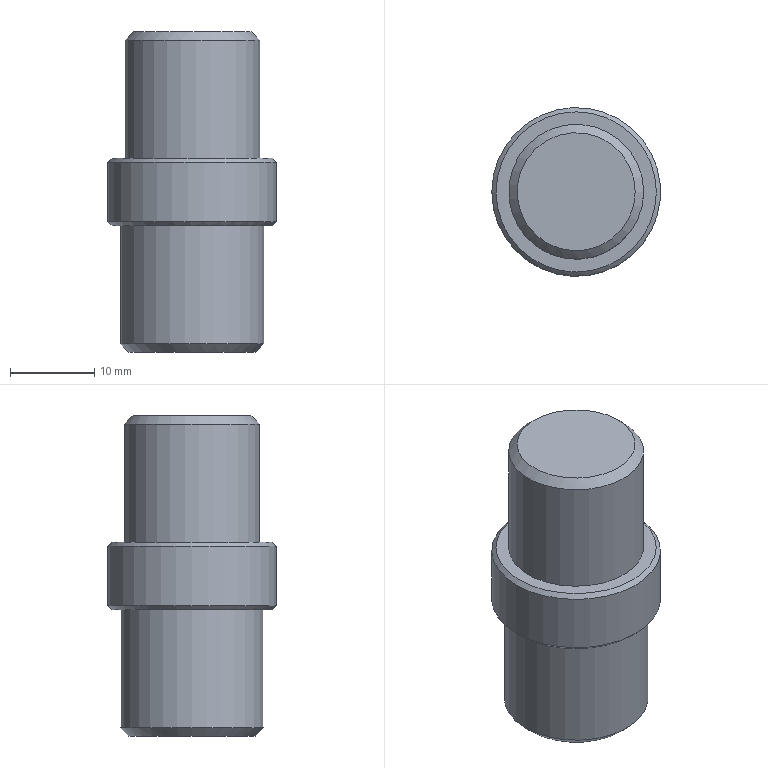Part | NX | features DATUM_CSYS 4, EXTRUDE 3, SKETCH 3, CHAMFER 2 | 1 solid | 11 faces | box 20 x 20 x 38 mm | volume 8869 mm3 | plane 4 | cone 4 | cylinder 3 | commonest cylinder face diameters 16 x1 17 x1 20 x1
STEP:
#1=CARTESIAN_POINT('',(8.,0.,14.));
#2=VERTEX_POINT('',#1);
#3=CARTESIAN_POINT('',(0.,0.,14.));
#4=DIRECTION('',(0.,0.,1.));
#5=DIRECTION('',(1.,0.,0.));
#6=AXIS2_PLACEMENT_3D('',#3,#4,#5);
#7=CIRCLE('',#6,8.);
#8=EDGE_CURVE('',#2,#2,#7,.F.);
#9=ORIENTED_EDGE('',*,*,#8,.T.);
#10=EDGE_LOOP('',(#9));
#11=FACE_BOUND('',#10,.T.);
#12=CARTESIAN_POINT('',(8.,0.,0.));
#13=VERTEX_POINT('',#12);
#14=CARTESIAN_POINT('',(0.,0.,0.));
#15=DIRECTION('',(0.,0.,1.));
#16=DIRECTION('',(1.,0.,0.));
#17=AXIS2_PLACEMENT_3D('',#14,#15,#16);
#18=CIRCLE('',#17,8.);
#19=EDGE_CURVE('',#13,#13,#18,.T.);
#20=ORIENTED_EDGE('',*,*,#19,.T.);
#21=EDGE_LOOP('',(#20));
#22=FACE_BOUND('',#21,.T.);
#23=CARTESIAN_POINT('',(0.,0.,15.));
#24=DIRECTION('',(0.,0.,-1.));
#25=DIRECTION('',(-1.,0.,0.));
#26=AXIS2_PLACEMENT_3D('',#23,#24,#25);
#27=CYLINDRICAL_SURFACE('',#26,8.);
#28=ADVANCED_FACE('',(#11,#22),#27,.T.);
#29=CARTESIAN_POINT('',(7.,0.,15.));
#30=VERTEX_POINT('',#29);
#31=CARTESIAN_POINT('',(0.,0.,15.));
#32=DIRECTION('',(0.,0.,1.));
#33=DIRECTION('',(1.,0.,0.));
#34=AXIS2_PLACEMENT_3D('',#31,#32,#33);
#35=CIRCLE('',#34,7.);
#36=EDGE_CURVE('',#30,#30,#35,.T.);
#37=ORIENTED_EDGE('',*,*,#36,.T.);
#38=EDGE_LOOP('',(#37));
#39=FACE_BOUND('',#38,.T.);
#40=CARTESIAN_POINT('',(0.,0.,15.));
#41=DIRECTION('',(0.,0.,1.));
#42=DIRECTION('',(1.,0.,0.));
#43=AXIS2_PLACEMENT_3D('',#40,#41,#42);
#44=PLANE('',#43);
#45=ADVANCED_FACE('',(#39),#44,.T.);
#46=CARTESIAN_POINT('',(-10.,0.,-7.5));
#47=VERTEX_POINT('',#46);
#48=CARTESIAN_POINT('',(0.,0.,-7.5));
#49=DIRECTION('',(0.,0.,-1.));
#50=DIRECTION('',(-1.,0.,0.));
#51=AXIS2_PLACEMENT_3D('',#48,#49,#50);
#52=CIRCLE('',#51,10.);
#53=EDGE_CURVE('',#47,#47,#52,.F.);
#54=ORIENTED_EDGE('',*,*,#53,.T.);
#55=EDGE_LOOP('',(#54));
#56=FACE_BOUND('',#55,.T.);
#57=CARTESIAN_POINT('',(-10.,0.,-0.5));
#58=VERTEX_POINT('',#57);
#59=CARTESIAN_POINT('',(0.,0.,-0.5));
#60=DIRECTION('',(0.,0.,-1.));
#61=DIRECTION('',(-1.,0.,0.));
#62=AXIS2_PLACEMENT_3D('',#59,#60,#61);
#63=CIRCLE('',#62,10.);
#64=EDGE_CURVE('',#58,#58,#63,.T.);
#65=ORIENTED_EDGE('',*,*,#64,.T.);
#66=EDGE_LOOP('',(#65));
#67=FACE_BOUND('',#66,.T.);
#68=CARTESIAN_POINT('',(0.,0.,-8.));
#69=DIRECTION('',(0.,0.,1.));
#70=DIRECTION('',(1.,0.,0.));
#71=AXIS2_PLACEMENT_3D('',#68,#69,#70);
#72=CYLINDRICAL_SURFACE('',#71,10.);
#73=ADVANCED_FACE('',(#56,#67),#72,.T.);
#74=CARTESIAN_POINT('',(-9.5,0.,-8.));
#75=VERTEX_POINT('',#74);
#76=CARTESIAN_POINT('',(0.,0.,-8.));
#77=DIRECTION('',(0.,0.,-1.));
#78=DIRECTION('',(-1.,0.,0.));
#79=AXIS2_PLACEMENT_3D('',#76,#77,#78);
#80=CIRCLE('',#79,9.5);
#81=EDGE_CURVE('',#75,#75,#80,.T.);
#82=ORIENTED_EDGE('',*,*,#81,.T.);
#83=EDGE_LOOP('',(#82));
#84=FACE_BOUND('',#83,.T.);
#85=CARTESIAN_POINT('',(8.5,0.,-8.));
#86=VERTEX_POINT('',#85);
#87=CARTESIAN_POINT('',(0.,0.,-8.));
#88=DIRECTION('',(0.,0.,-1.));
#89=DIRECTION('',(1.,0.,0.));
#90=AXIS2_PLACEMENT_3D('',#87,#88,#89);
#91=CIRCLE('',#90,8.5);
#92=EDGE_CURVE('',#86,#86,#91,.T.);
#93=ORIENTED_EDGE('',*,*,#92,.F.);
#94=EDGE_LOOP('',(#93));
#95=FACE_BOUND('',#94,.T.);
#96=CARTESIAN_POINT('',(0.,0.,-8.));
#97=DIRECTION('',(0.,0.,-1.));
#98=DIRECTION('',(-1.,0.,0.));
#99=AXIS2_PLACEMENT_3D('',#96,#97,#98);
#100=PLANE('',#99);
#101=ADVANCED_FACE('',(#84,#95),#100,.T.);
#102=CARTESIAN_POINT('',(-9.5,0.,0.));
#103=VERTEX_POINT('',#102);
#104=CARTESIAN_POINT('',(0.,0.,0.));
#105=DIRECTION('',(0.,0.,-1.));
#106=DIRECTION('',(-1.,0.,0.));
#107=AXIS2_PLACEMENT_3D('',#104,#105,#106);
#108=CIRCLE('',#107,9.5);
#109=EDGE_CURVE('',#103,#103,#108,.F.);
#110=ORIENTED_EDGE('',*,*,#109,.T.);
#111=EDGE_LOOP('',(#110));
#112=FACE_BOUND('',#111,.T.);
#113=ORIENTED_EDGE('',*,*,#19,.F.);
#114=EDGE_LOOP('',(#113));
#115=FACE_BOUND('',#114,.T.);
#116=CARTESIAN_POINT('',(0.,0.,0.));
#117=DIRECTION('',(0.,0.,-1.));
#118=DIRECTION('',(-1.,0.,0.));
#119=AXIS2_PLACEMENT_3D('',#116,#117,#118);
#120=PLANE('',#119);
#121=ADVANCED_FACE('',(#112,#115),#120,.F.);
#122=CARTESIAN_POINT('',(-8.5,0.,-22.));
#123=VERTEX_POINT('',#122);
#124=CARTESIAN_POINT('',(0.,0.,-22.));
#125=DIRECTION('',(0.,0.,-1.));
#126=DIRECTION('',(-1.,0.,0.));
#127=AXIS2_PLACEMENT_3D('',#124,#125,#126);
#128=CIRCLE('',#127,8.5);
#129=EDGE_CURVE('',#123,#123,#128,.F.);
#130=ORIENTED_EDGE('',*,*,#129,.T.);
#131=EDGE_LOOP('',(#130));
#132=FACE_BOUND('',#131,.T.);
#133=ORIENTED_EDGE('',*,*,#92,.T.);
#134=EDGE_LOOP('',(#133));
#135=FACE_BOUND('',#134,.T.);
#136=CARTESIAN_POINT('',(0.,0.,-23.));
#137=DIRECTION('',(0.,0.,1.));
#138=DIRECTION('',(1.,0.,0.));
#139=AXIS2_PLACEMENT_3D('',#136,#137,#138);
#140=CYLINDRICAL_SURFACE('',#139,8.5);
#141=ADVANCED_FACE('',(#132,#135),#140,.T.);
#142=CARTESIAN_POINT('',(-7.5,0.,-23.));
#143=VERTEX_POINT('',#142);
#144=CARTESIAN_POINT('',(0.,0.,-23.));
#145=DIRECTION('',(0.,0.,-1.));
#146=DIRECTION('',(-1.,0.,0.));
#147=AXIS2_PLACEMENT_3D('',#144,#145,#146);
#148=CIRCLE('',#147,7.5);
#149=EDGE_CURVE('',#143,#143,#148,.T.);
#150=ORIENTED_EDGE('',*,*,#149,.T.);
#151=EDGE_LOOP('',(#150));
#152=FACE_BOUND('',#151,.T.);
#153=CARTESIAN_POINT('',(0.,0.,-23.));
#154=DIRECTION('',(0.,0.,-1.));
#155=DIRECTION('',(-1.,0.,0.));
#156=AXIS2_PLACEMENT_3D('',#153,#154,#155);
#157=PLANE('',#156);
#158=ADVANCED_FACE('',(#152),#157,.T.);
#159=ORIENTED_EDGE('',*,*,#129,.F.);
#160=EDGE_LOOP('',(#159));
#161=FACE_BOUND('',#160,.T.);
#162=ORIENTED_EDGE('',*,*,#149,.F.);
#163=EDGE_LOOP('',(#162));
#164=FACE_BOUND('',#163,.T.);
#165=CARTESIAN_POINT('',(0.,0.,-23.));
#166=DIRECTION('',(0.,0.,1.));
#167=DIRECTION('',(1.,0.,0.));
#168=AXIS2_PLACEMENT_3D('',#165,#166,#167);
#169=CONICAL_SURFACE('',#168,7.5,0.7854);
#170=ADVANCED_FACE('',(#161,#164),#169,.T.);
#171=ORIENTED_EDGE('',*,*,#8,.F.);
#172=EDGE_LOOP('',(#171));
#173=FACE_BOUND('',#172,.T.);
#174=ORIENTED_EDGE('',*,*,#36,.F.);
#175=EDGE_LOOP('',(#174));
#176=FACE_BOUND('',#175,.T.);
#177=CARTESIAN_POINT('',(0.,0.,15.));
#178=DIRECTION('',(0.,0.,-1.));
#179=DIRECTION('',(-1.,0.,0.));
#180=AXIS2_PLACEMENT_3D('',#177,#178,#179);
#181=CONICAL_SURFACE('',#180,7.,0.7854);
#182=ADVANCED_FACE('',(#173,#176),#181,.T.);
#183=ORIENTED_EDGE('',*,*,#53,.F.);
#184=EDGE_LOOP('',(#183));
#185=FACE_BOUND('',#184,.T.);
#186=ORIENTED_EDGE('',*,*,#81,.F.);
#187=EDGE_LOOP('',(#186));
#188=FACE_BOUND('',#187,.T.);
#189=CARTESIAN_POINT('',(0.,0.,-8.));
#190=DIRECTION('',(0.,0.,1.));
#191=DIRECTION('',(1.,0.,0.));
#192=AXIS2_PLACEMENT_3D('',#189,#190,#191);
#193=CONICAL_SURFACE('',#192,9.5,0.7854);
#194=ADVANCED_FACE('',(#185,#188),#193,.T.);
#195=ORIENTED_EDGE('',*,*,#109,.F.);
#196=EDGE_LOOP('',(#195));
#197=FACE_BOUND('',#196,.T.);
#198=ORIENTED_EDGE('',*,*,#64,.F.);
#199=EDGE_LOOP('',(#198));
#200=FACE_BOUND('',#199,.T.);
#201=CARTESIAN_POINT('',(0.,0.,-0.5));
#202=DIRECTION('',(0.,0.,-1.));
#203=DIRECTION('',(-1.,0.,0.));
#204=AXIS2_PLACEMENT_3D('',#201,#202,#203);
#205=CONICAL_SURFACE('',#204,10.,0.7854);
#206=ADVANCED_FACE('',(#197,#200),#205,.T.);
#207=CLOSED_SHELL('',(#28,#45,#73,#101,#121,#141,#158,#170,#182,#194,#206));
#208=MANIFOLD_SOLID_BREP('',#207);
#209=(LENGTH_UNIT()NAMED_UNIT(*)SI_UNIT(.MILLI.,.METRE.));
#210=UNCERTAINTY_MEASURE_WITH_UNIT(LENGTH_MEASURE(0.00001),#209,'','');
#211=(NAMED_UNIT(*)PLANE_ANGLE_UNIT()SI_UNIT($,.RADIAN.));
#212=(NAMED_UNIT(*)SI_UNIT($,.STERADIAN.)SOLID_ANGLE_UNIT());
#213=(GEOMETRIC_REPRESENTATION_CONTEXT(3)GLOBAL_UNCERTAINTY_ASSIGNED_CONTEXT((#210))GLOBAL_UNIT_ASSIGNED_CONTEXT((#209,#211,#212))REPRESENTATION_CONTEXT('',''));
#214=ADVANCED_BREP_SHAPE_REPRESENTATION('',(#208),#213);